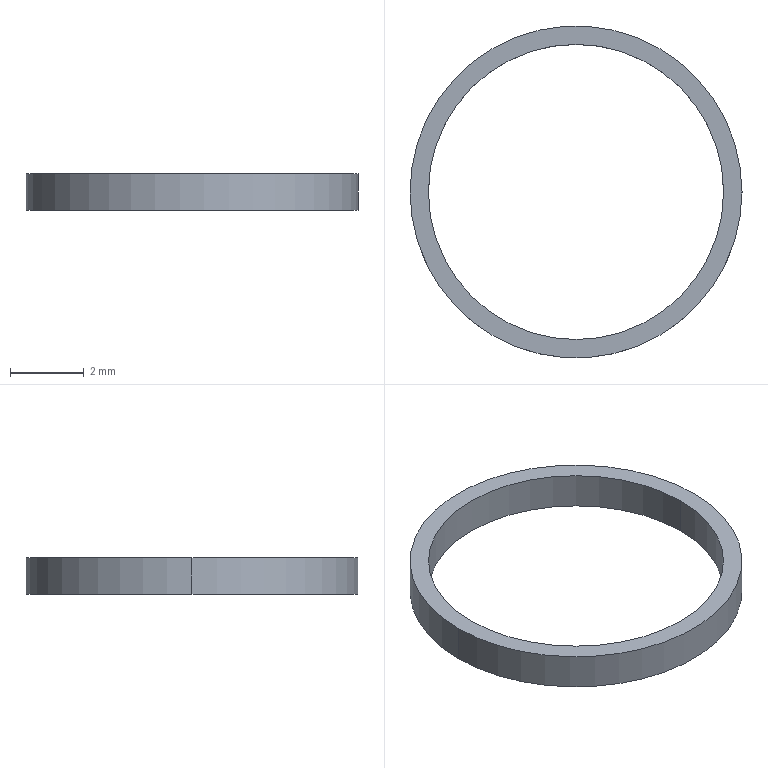Part | SolidWorks | features Extrusion 1 | 1 solid | 6 faces | box 9 x 9 x 1 mm | volume 13.352 mm3 | cylinder 4 | plane 2 | commonest cylinder face diameters 8 x2 9 x2
STEP:
#1=CARTESIAN_POINT('',(-4.,0.,1.));
#2=VERTEX_POINT('',#1);
#3=CARTESIAN_POINT('',(4.,0.,1.));
#4=VERTEX_POINT('',#3);
#5=CARTESIAN_POINT('',(0.,0.,1.));
#6=DIRECTION('',(0.,0.,1.));
#7=DIRECTION('',(1.,0.,0.));
#8=AXIS2_PLACEMENT_3D('',#5,#6,#7);
#9=CIRCLE('',#8,4.);
#10=EDGE_CURVE('',#2,#4,#9,.T.);
#11=ORIENTED_EDGE('',*,*,#10,.T.);
#12=CARTESIAN_POINT('',(4.,0.,0.));
#13=VERTEX_POINT('',#12);
#14=CARTESIAN_POINT('',(4.,0.,1.));
#15=DIRECTION('',(0.,0.,-1.));
#16=VECTOR('',#15,1000.);
#17=LINE('',#14,#16);
#18=EDGE_CURVE('',#4,#13,#17,.T.);
#19=ORIENTED_EDGE('',*,*,#18,.T.);
#20=CARTESIAN_POINT('',(-4.,0.,0.));
#21=VERTEX_POINT('',#20);
#22=CARTESIAN_POINT('',(0.,0.,0.));
#23=DIRECTION('',(0.,0.,1.));
#24=DIRECTION('',(1.,0.,0.));
#25=AXIS2_PLACEMENT_3D('',#22,#23,#24);
#26=CIRCLE('',#25,4.);
#27=EDGE_CURVE('',#21,#13,#26,.T.);
#28=ORIENTED_EDGE('',*,*,#27,.F.);
#29=CARTESIAN_POINT('',(-4.,0.,1.));
#30=DIRECTION('',(0.,0.,-1.));
#31=VECTOR('',#30,1000.);
#32=LINE('',#29,#31);
#33=EDGE_CURVE('',#2,#21,#32,.T.);
#34=ORIENTED_EDGE('',*,*,#33,.F.);
#35=EDGE_LOOP('',(#11,#19,#28,#34));
#36=FACE_OUTER_BOUND('',#35,.T.);
#37=CARTESIAN_POINT('',(0.,0.,1.));
#38=DIRECTION('',(0.,0.,-1.));
#39=DIRECTION('',(-1.,0.,0.));
#40=AXIS2_PLACEMENT_3D('',#37,#38,#39);
#41=CYLINDRICAL_SURFACE('',#40,4.);
#42=ADVANCED_FACE('',(#36),#41,.F.);
#43=CARTESIAN_POINT('',(4.5,0.,1.));
#44=VERTEX_POINT('',#43);
#45=CARTESIAN_POINT('',(-4.5,0.,1.));
#46=VERTEX_POINT('',#45);
#47=CARTESIAN_POINT('',(0.,0.,1.));
#48=DIRECTION('',(0.,0.,1.));
#49=DIRECTION('',(1.,0.,0.));
#50=AXIS2_PLACEMENT_3D('',#47,#48,#49);
#51=CIRCLE('',#50,4.5);
#52=EDGE_CURVE('',#44,#46,#51,.T.);
#53=ORIENTED_EDGE('',*,*,#52,.F.);
#54=CARTESIAN_POINT('',(4.5,0.,0.));
#55=VERTEX_POINT('',#54);
#56=CARTESIAN_POINT('',(4.5,0.,1.));
#57=DIRECTION('',(0.,0.,-1.));
#58=VECTOR('',#57,1000.);
#59=LINE('',#56,#58);
#60=EDGE_CURVE('',#44,#55,#59,.T.);
#61=ORIENTED_EDGE('',*,*,#60,.T.);
#62=CARTESIAN_POINT('',(-4.5,0.,0.));
#63=VERTEX_POINT('',#62);
#64=CARTESIAN_POINT('',(0.,0.,0.));
#65=DIRECTION('',(0.,0.,1.));
#66=DIRECTION('',(1.,0.,0.));
#67=AXIS2_PLACEMENT_3D('',#64,#65,#66);
#68=CIRCLE('',#67,4.5);
#69=EDGE_CURVE('',#55,#63,#68,.T.);
#70=ORIENTED_EDGE('',*,*,#69,.T.);
#71=CARTESIAN_POINT('',(-4.5,0.,1.));
#72=DIRECTION('',(0.,0.,-1.));
#73=VECTOR('',#72,1000.);
#74=LINE('',#71,#73);
#75=EDGE_CURVE('',#46,#63,#74,.T.);
#76=ORIENTED_EDGE('',*,*,#75,.F.);
#77=EDGE_LOOP('',(#53,#61,#70,#76));
#78=FACE_OUTER_BOUND('',#77,.T.);
#79=CARTESIAN_POINT('',(0.,0.,1.));
#80=DIRECTION('',(0.,0.,-1.));
#81=DIRECTION('',(-1.,0.,0.));
#82=AXIS2_PLACEMENT_3D('',#79,#80,#81);
#83=CYLINDRICAL_SURFACE('',#82,4.5);
#84=ADVANCED_FACE('',(#78),#83,.T.);
#85=CARTESIAN_POINT('',(0.,0.,1.));
#86=DIRECTION('',(0.,0.,1.));
#87=DIRECTION('',(1.,0.,0.));
#88=AXIS2_PLACEMENT_3D('',#85,#86,#87);
#89=CIRCLE('',#88,4.5);
#90=EDGE_CURVE('',#46,#44,#89,.T.);
#91=ORIENTED_EDGE('',*,*,#90,.T.);
#92=ORIENTED_EDGE('',*,*,#52,.T.);
#93=EDGE_LOOP('',(#91,#92));
#94=FACE_OUTER_BOUND('',#93,.T.);
#95=ORIENTED_EDGE('',*,*,#10,.F.);
#96=CARTESIAN_POINT('',(0.,0.,1.));
#97=DIRECTION('',(0.,0.,1.));
#98=DIRECTION('',(1.,0.,0.));
#99=AXIS2_PLACEMENT_3D('',#96,#97,#98);
#100=CIRCLE('',#99,4.);
#101=EDGE_CURVE('',#4,#2,#100,.T.);
#102=ORIENTED_EDGE('',*,*,#101,.F.);
#103=EDGE_LOOP('',(#95,#102));
#104=FACE_BOUND('',#103,.T.);
#105=CARTESIAN_POINT('',(0.,0.,1.));
#106=DIRECTION('',(0.,0.,1.));
#107=DIRECTION('',(1.,0.,0.));
#108=AXIS2_PLACEMENT_3D('',#105,#106,#107);
#109=PLANE('',#108);
#110=ADVANCED_FACE('',(#94,#104),#109,.T.);
#111=CARTESIAN_POINT('',(0.,0.,0.));
#112=DIRECTION('',(0.,0.,1.));
#113=DIRECTION('',(1.,0.,0.));
#114=AXIS2_PLACEMENT_3D('',#111,#112,#113);
#115=CIRCLE('',#114,4.5);
#116=EDGE_CURVE('',#63,#55,#115,.T.);
#117=ORIENTED_EDGE('',*,*,#116,.F.);
#118=ORIENTED_EDGE('',*,*,#69,.F.);
#119=EDGE_LOOP('',(#117,#118));
#120=FACE_OUTER_BOUND('',#119,.T.);
#121=ORIENTED_EDGE('',*,*,#27,.T.);
#122=CARTESIAN_POINT('',(0.,0.,0.));
#123=DIRECTION('',(0.,0.,1.));
#124=DIRECTION('',(1.,0.,0.));
#125=AXIS2_PLACEMENT_3D('',#122,#123,#124);
#126=CIRCLE('',#125,4.);
#127=EDGE_CURVE('',#13,#21,#126,.T.);
#128=ORIENTED_EDGE('',*,*,#127,.T.);
#129=EDGE_LOOP('',(#121,#128));
#130=FACE_BOUND('',#129,.T.);
#131=CARTESIAN_POINT('',(0.,0.,0.));
#132=DIRECTION('',(0.,0.,1.));
#133=DIRECTION('',(1.,0.,0.));
#134=AXIS2_PLACEMENT_3D('',#131,#132,#133);
#135=PLANE('',#134);
#136=ADVANCED_FACE('',(#120,#130),#135,.F.);
#137=ORIENTED_EDGE('',*,*,#60,.F.);
#138=ORIENTED_EDGE('',*,*,#90,.F.);
#139=ORIENTED_EDGE('',*,*,#75,.T.);
#140=ORIENTED_EDGE('',*,*,#116,.T.);
#141=EDGE_LOOP('',(#137,#138,#139,#140));
#142=FACE_OUTER_BOUND('',#141,.T.);
#143=CARTESIAN_POINT('',(0.,0.,1.));
#144=DIRECTION('',(0.,0.,-1.));
#145=DIRECTION('',(-1.,0.,0.));
#146=AXIS2_PLACEMENT_3D('',#143,#144,#145);
#147=CYLINDRICAL_SURFACE('',#146,4.5);
#148=ADVANCED_FACE('',(#142),#147,.T.);
#149=ORIENTED_EDGE('',*,*,#18,.F.);
#150=ORIENTED_EDGE('',*,*,#101,.T.);
#151=ORIENTED_EDGE('',*,*,#33,.T.);
#152=ORIENTED_EDGE('',*,*,#127,.F.);
#153=EDGE_LOOP('',(#149,#150,#151,#152));
#154=FACE_OUTER_BOUND('',#153,.T.);
#155=CARTESIAN_POINT('',(0.,0.,1.));
#156=DIRECTION('',(0.,0.,-1.));
#157=DIRECTION('',(-1.,0.,0.));
#158=AXIS2_PLACEMENT_3D('',#155,#156,#157);
#159=CYLINDRICAL_SURFACE('',#158,4.);
#160=ADVANCED_FACE('',(#154),#159,.F.);
#161=CLOSED_SHELL('',(#42,#84,#110,#136,#148,#160));
#162=MANIFOLD_SOLID_BREP('',#161);
#163=CARTESIAN_POINT('',(0.,0.,0.));
#164=DIRECTION('',(0.,0.,1.));
#165=DIRECTION('',(1.,0.,0.));
#166=AXIS2_PLACEMENT_3D('',#163,#164,#165);
#167=(LENGTH_UNIT()NAMED_UNIT(*)SI_UNIT(.MILLI.,.METRE.));
#168=UNCERTAINTY_MEASURE_WITH_UNIT(LENGTH_MEASURE(0.00001),#167,'','');
#169=(NAMED_UNIT(*)PLANE_ANGLE_UNIT()SI_UNIT($,.RADIAN.));
#170=(NAMED_UNIT(*)SI_UNIT($,.STERADIAN.)SOLID_ANGLE_UNIT());
#171=(GEOMETRIC_REPRESENTATION_CONTEXT(3)GLOBAL_UNCERTAINTY_ASSIGNED_CONTEXT((#168))GLOBAL_UNIT_ASSIGNED_CONTEXT((#167,#169,#170))REPRESENTATION_CONTEXT('',''));
#172=ADVANCED_BREP_SHAPE_REPRESENTATION('',(#162,#166),#171);